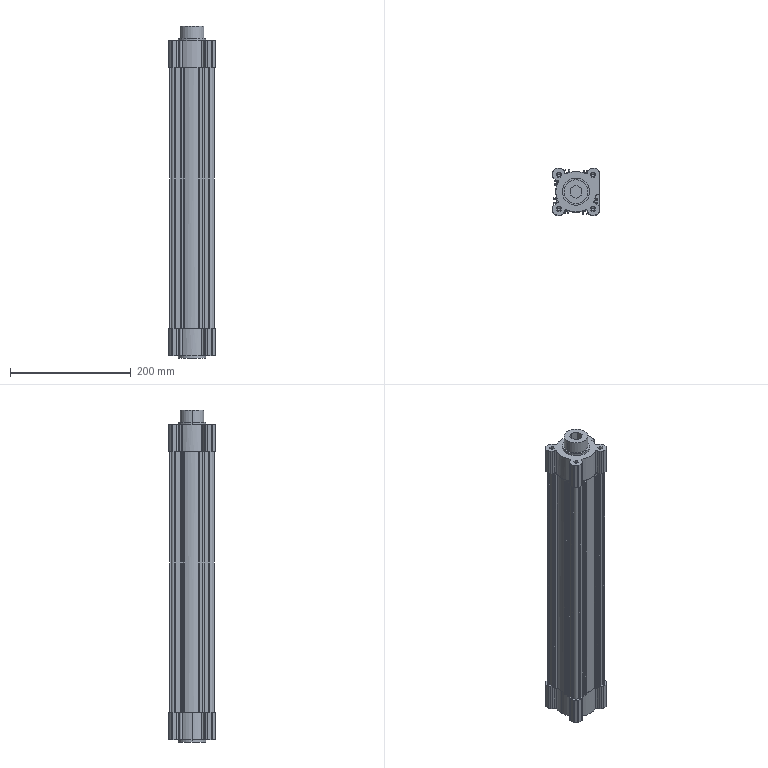Part | SolidWorks | features BaseBody 1 | 1 solid | 427 faces | box 77 x 77 x 549 mm | volume 1151888 mm3 | plane 259 | cylinder 128 | cone 40 | commonest cylinder face diameters 8 x30 4 x17 6.647 x16 20 x14 4.25 x9 67 x9